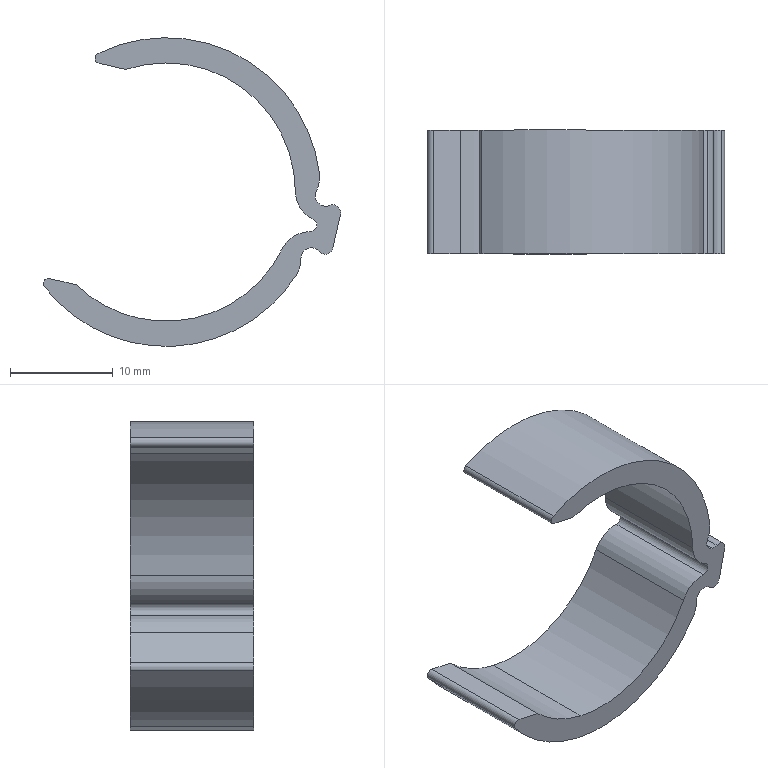Part | SolidWorks | features BaseBody 1 | 1 solid | 25 faces | box 28.907 x 12 x 30 mm | volume 1841 mm3 | cylinder 20 | plane 5 | commonest cylinder face diameters 6 x4 2 x3 25.1 x3 30 x3 1 x2 1.5 x2
STEP:
#1=CARTESIAN_POINT('',(1964.27,-217.65,847.477));
#2=VERTEX_POINT('',#1);
#3=CARTESIAN_POINT('',(1950.19,-217.65,840.769));
#4=VERTEX_POINT('',#3);
#5=CARTESIAN_POINT('',(1953.,-217.65,853.));
#6=DIRECTION('',(0.,1.,0.));
#7=DIRECTION('',(0.898,0.,-0.4401));
#8=AXIS2_PLACEMENT_3D('',#5,#6,#7);
#9=CIRCLE('',#8,12.55);
#10=EDGE_CURVE('',#2,#4,#9,.T.);
#11=ORIENTED_EDGE('',*,*,#10,.T.);
#12=CARTESIAN_POINT('',(1950.19,-229.65,840.769));
#13=VERTEX_POINT('',#12);
#14=CARTESIAN_POINT('',(1950.19,-217.65,840.769));
#15=DIRECTION('',(0.,-1.,0.));
#16=VECTOR('',#15,1000.);
#17=LINE('',#14,#16);
#18=EDGE_CURVE('',#4,#13,#17,.T.);
#19=ORIENTED_EDGE('',*,*,#18,.T.);
#20=CARTESIAN_POINT('',(1964.27,-229.65,847.477));
#21=VERTEX_POINT('',#20);
#22=CARTESIAN_POINT('',(1953.,-229.65,853.));
#23=DIRECTION('',(0.,1.,0.));
#24=DIRECTION('',(0.898,0.,-0.4401));
#25=AXIS2_PLACEMENT_3D('',#22,#23,#24);
#26=CIRCLE('',#25,12.55);
#27=EDGE_CURVE('',#21,#13,#26,.T.);
#28=ORIENTED_EDGE('',*,*,#27,.F.);
#29=CARTESIAN_POINT('',(1964.27,-229.65,847.477));
#30=DIRECTION('',(0.,1.,0.));
#31=VECTOR('',#30,1000.);
#32=LINE('',#29,#31);
#33=EDGE_CURVE('',#21,#2,#32,.T.);
#34=ORIENTED_EDGE('',*,*,#33,.T.);
#35=EDGE_LOOP('',(#11,#19,#28,#34));
#36=FACE_OUTER_BOUND('',#35,.T.);
#37=CARTESIAN_POINT('',(1953.,-217.65,853.));
#38=DIRECTION('',(0.,-1.,0.));
#39=DIRECTION('',(-0.2239,0.,-0.9746));
#40=AXIS2_PLACEMENT_3D('',#37,#38,#39);
#41=CYLINDRICAL_SURFACE('',#40,12.55);
#42=ADVANCED_FACE('',(#36),#41,.F.);
#43=CARTESIAN_POINT('',(1941.157,-217.65,843.795));
#44=VERTEX_POINT('',#43);
#45=CARTESIAN_POINT('',(1949.642,-217.65,838.381));
#46=VERTEX_POINT('',#45);
#47=CARTESIAN_POINT('',(1953.,-217.65,853.));
#48=DIRECTION('',(0.,-1.,0.));
#49=DIRECTION('',(-0.7895,0.,-0.6137));
#50=AXIS2_PLACEMENT_3D('',#47,#48,#49);
#51=CIRCLE('',#50,15.);
#52=EDGE_CURVE('',#44,#46,#51,.T.);
#53=ORIENTED_EDGE('',*,*,#52,.T.);
#54=CARTESIAN_POINT('',(1949.642,-229.65,838.381));
#55=VERTEX_POINT('',#54);
#56=CARTESIAN_POINT('',(1949.642,-217.65,838.381));
#57=DIRECTION('',(0.,-1.,0.));
#58=VECTOR('',#57,1000.);
#59=LINE('',#56,#58);
#60=EDGE_CURVE('',#46,#55,#59,.T.);
#61=ORIENTED_EDGE('',*,*,#60,.T.);
#62=CARTESIAN_POINT('',(1941.157,-229.65,843.795));
#63=VERTEX_POINT('',#62);
#64=CARTESIAN_POINT('',(1953.,-229.65,853.));
#65=DIRECTION('',(0.,-1.,0.));
#66=DIRECTION('',(-0.7895,0.,-0.6137));
#67=AXIS2_PLACEMENT_3D('',#64,#65,#66);
#68=CIRCLE('',#67,15.);
#69=EDGE_CURVE('',#63,#55,#68,.T.);
#70=ORIENTED_EDGE('',*,*,#69,.F.);
#71=CARTESIAN_POINT('',(1941.157,-229.65,843.795));
#72=DIRECTION('',(0.,1.,0.));
#73=VECTOR('',#72,1000.);
#74=LINE('',#71,#73);
#75=EDGE_CURVE('',#63,#44,#74,.T.);
#76=ORIENTED_EDGE('',*,*,#75,.T.);
#77=EDGE_LOOP('',(#53,#61,#70,#76));
#78=FACE_OUTER_BOUND('',#77,.T.);
#79=CARTESIAN_POINT('',(1953.,-217.65,853.));
#80=DIRECTION('',(0.,-1.,0.));
#81=DIRECTION('',(-0.2239,0.,-0.9746));
#82=AXIS2_PLACEMENT_3D('',#79,#80,#81);
#83=CYLINDRICAL_SURFACE('',#82,15.);
#84=ADVANCED_FACE('',(#78),#83,.T.);
#85=CARTESIAN_POINT('',(1968.258,-217.65,851.649));
#86=VERTEX_POINT('',#85);
#87=CARTESIAN_POINT('',(1968.885,-217.65,851.709));
#88=VERTEX_POINT('',#87);
#89=CARTESIAN_POINT('',(1968.482,-217.65,852.624));
#90=DIRECTION('',(0.,-1.,0.));
#91=DIRECTION('',(-0.892,0.,0.452));
#92=AXIS2_PLACEMENT_3D('',#89,#90,#91);
#93=CIRCLE('',#92,1.);
#94=EDGE_CURVE('',#86,#88,#93,.T.);
#95=ORIENTED_EDGE('',*,*,#94,.F.);
#96=CARTESIAN_POINT('',(1968.258,-229.65,851.649));
#97=VERTEX_POINT('',#96);
#98=CARTESIAN_POINT('',(1968.258,-230.85,851.649));
#99=DIRECTION('',(0.,-1.,0.));
#100=VECTOR('',#99,1000.);
#101=LINE('',#98,#100);
#102=EDGE_CURVE('',#86,#97,#101,.T.);
#103=ORIENTED_EDGE('',*,*,#102,.T.);
#104=CARTESIAN_POINT('',(1968.885,-229.65,851.709));
#105=VERTEX_POINT('',#104);
#106=CARTESIAN_POINT('',(1968.482,-229.65,852.624));
#107=DIRECTION('',(0.,1.,0.));
#108=DIRECTION('',(0.4028,0.,-0.9153));
#109=AXIS2_PLACEMENT_3D('',#106,#107,#108);
#110=CIRCLE('',#109,1.);
#111=EDGE_CURVE('',#105,#97,#110,.T.);
#112=ORIENTED_EDGE('',*,*,#111,.F.);
#113=CARTESIAN_POINT('',(1968.885,-217.65,851.709));
#114=DIRECTION('',(0.,-1.,0.));
#115=VECTOR('',#114,1000.);
#116=LINE('',#113,#115);
#117=EDGE_CURVE('',#88,#105,#116,.T.);
#118=ORIENTED_EDGE('',*,*,#117,.F.);
#119=EDGE_LOOP('',(#95,#103,#112,#118));
#120=FACE_OUTER_BOUND('',#119,.T.);
#121=CARTESIAN_POINT('',(1968.482,-230.85,852.624));
#122=DIRECTION('',(0.,-1.,0.));
#123=DIRECTION('',(-0.2239,0.,-0.9746));
#124=AXIS2_PLACEMENT_3D('',#121,#122,#123);
#125=CYLINDRICAL_SURFACE('',#124,1.);
#126=ADVANCED_FACE('',(#120),#125,.F.);
#127=CARTESIAN_POINT('',(1969.622,-217.65,851.633));
#128=VERTEX_POINT('',#127);
#129=CARTESIAN_POINT('',(1969.187,-217.65,851.022));
#130=DIRECTION('',(0.,1.,0.));
#131=DIRECTION('',(-0.4028,0.,0.9153));
#132=AXIS2_PLACEMENT_3D('',#129,#130,#131);
#133=CIRCLE('',#132,0.75);
#134=EDGE_CURVE('',#88,#128,#133,.T.);
#135=ORIENTED_EDGE('',*,*,#134,.T.);
#136=CARTESIAN_POINT('',(1969.938,-217.65,850.802));
#137=VERTEX_POINT('',#136);
#138=CARTESIAN_POINT('',(1969.158,-217.65,850.981));
#139=DIRECTION('',(0.,1.,0.));
#140=DIRECTION('',(0.5796,0.,0.8149));
#141=AXIS2_PLACEMENT_3D('',#138,#139,#140);
#142=CIRCLE('',#141,0.8);
#143=EDGE_CURVE('',#128,#137,#142,.T.);
#144=ORIENTED_EDGE('',*,*,#143,.T.);
#145=CARTESIAN_POINT('',(1969.199,-217.65,847.586));
#146=VERTEX_POINT('',#145);
#147=CARTESIAN_POINT('',(1969.199,-217.65,847.586));
#148=DIRECTION('',(0.2239,0.,0.9746));
#149=VECTOR('',#148,1000.);
#150=LINE('',#147,#149);
#151=EDGE_CURVE('',#146,#137,#150,.T.);
#152=ORIENTED_EDGE('',*,*,#151,.F.);
#153=CARTESIAN_POINT('',(1968.552,-217.65,846.976));
#154=VERTEX_POINT('',#153);
#155=CARTESIAN_POINT('',(1968.419,-217.65,847.765));
#156=DIRECTION('',(0.,1.,0.));
#157=DIRECTION('',(0.9746,0.,-0.2239));
#158=AXIS2_PLACEMENT_3D('',#155,#156,#157);
#159=CIRCLE('',#158,0.8);
#160=EDGE_CURVE('',#146,#154,#159,.T.);
#161=ORIENTED_EDGE('',*,*,#160,.T.);
#162=CARTESIAN_POINT('',(1967.856,-217.65,847.23));
#163=VERTEX_POINT('',#162);
#164=CARTESIAN_POINT('',(1968.428,-217.65,847.716));
#165=DIRECTION('',(0.,1.,0.));
#166=DIRECTION('',(0.1659,0.,-0.9861));
#167=AXIS2_PLACEMENT_3D('',#164,#165,#166);
#168=CIRCLE('',#167,0.75);
#169=EDGE_CURVE('',#154,#163,#168,.T.);
#170=ORIENTED_EDGE('',*,*,#169,.T.);
#171=CARTESIAN_POINT('',(1966.095,-217.65,846.565));
#172=VERTEX_POINT('',#171);
#173=CARTESIAN_POINT('',(1967.095,-217.65,846.582));
#174=DIRECTION('',(0.,-1.,0.));
#175=DIRECTION('',(0.7618,0.,0.6478));
#176=AXIS2_PLACEMENT_3D('',#173,#174,#175);
#177=CIRCLE('',#176,1.);
#178=EDGE_CURVE('',#163,#172,#177,.T.);
#179=ORIENTED_EDGE('',*,*,#178,.T.);
#180=CARTESIAN_POINT('',(1965.619,-217.65,844.891));
#181=VERTEX_POINT('',#180);
#182=CARTESIAN_POINT('',(1963.095,-217.65,846.513));
#183=DIRECTION('',(0.,1.,0.));
#184=DIRECTION('',(0.9998,0.,0.01744));
#185=AXIS2_PLACEMENT_3D('',#182,#183,#184);
#186=CIRCLE('',#185,3.);
#187=EDGE_CURVE('',#172,#181,#186,.T.);
#188=ORIENTED_EDGE('',*,*,#187,.T.);
#189=CARTESIAN_POINT('',(1953.,-217.65,853.));
#190=DIRECTION('',(0.,-1.,0.));
#191=DIRECTION('',(-0.7895,0.,-0.6137));
#192=AXIS2_PLACEMENT_3D('',#189,#190,#191);
#193=CIRCLE('',#192,15.);
#194=EDGE_CURVE('',#46,#181,#193,.T.);
#195=ORIENTED_EDGE('',*,*,#194,.F.);
#196=ORIENTED_EDGE('',*,*,#52,.F.);
#197=CARTESIAN_POINT('',(1941.663,-217.65,844.589));
#198=VERTEX_POINT('',#197);
#199=CARTESIAN_POINT('',(1941.552,-217.65,844.102));
#200=DIRECTION('',(0.,1.,0.));
#201=DIRECTION('',(-0.7895,0.,-0.6137));
#202=AXIS2_PLACEMENT_3D('',#199,#200,#201);
#203=CIRCLE('',#202,0.5);
#204=EDGE_CURVE('',#44,#198,#203,.T.);
#205=ORIENTED_EDGE('',*,*,#204,.T.);
#206=CARTESIAN_POINT('',(1944.262,-217.65,843.992));
#207=VERTEX_POINT('',#206);
#208=CARTESIAN_POINT('',(1944.262,-217.65,843.992));
#209=DIRECTION('',(-0.9746,0.,0.2239));
#210=VECTOR('',#209,1000.);
#211=LINE('',#208,#210);
#212=EDGE_CURVE('',#207,#198,#211,.T.);
#213=ORIENTED_EDGE('',*,*,#212,.F.);
#214=CARTESIAN_POINT('',(1953.,-217.65,853.));
#215=DIRECTION('',(0.,1.,0.));
#216=DIRECTION('',(0.898,0.,-0.4401));
#217=AXIS2_PLACEMENT_3D('',#214,#215,#216);
#218=CIRCLE('',#217,12.55);
#219=EDGE_CURVE('',#4,#207,#218,.T.);
#220=ORIENTED_EDGE('',*,*,#219,.F.);
#221=ORIENTED_EDGE('',*,*,#10,.F.);
#222=CARTESIAN_POINT('',(1967.002,-217.65,849.157));
#223=VERTEX_POINT('',#222);
#224=CARTESIAN_POINT('',(1966.963,-217.65,846.157));
#225=DIRECTION('',(0.,1.,0.));
#226=DIRECTION('',(-0.898,0.,0.4401));
#227=AXIS2_PLACEMENT_3D('',#224,#225,#226);
#228=CIRCLE('',#227,3.);
#229=EDGE_CURVE('',#2,#223,#228,.T.);
#230=ORIENTED_EDGE('',*,*,#229,.T.);
#231=CARTESIAN_POINT('',(1967.276,-217.65,850.348));
#232=VERTEX_POINT('',#231);
#233=CARTESIAN_POINT('',(1967.01,-217.65,849.782));
#234=DIRECTION('',(0.,-1.,0.));
#235=DIRECTION('',(-0.01288,0.,-0.9999));
#236=AXIS2_PLACEMENT_3D('',#233,#234,#235);
#237=CIRCLE('',#236,0.625);
#238=EDGE_CURVE('',#223,#232,#237,.T.);
#239=ORIENTED_EDGE('',*,*,#238,.T.);
#240=CARTESIAN_POINT('',(1965.55,-217.65,853.051));
#241=VERTEX_POINT('',#240);
#242=CARTESIAN_POINT('',(1968.55,-217.65,853.064));
#243=DIRECTION('',(0.,1.,0.));
#244=DIRECTION('',(-0.4247,0.,-0.9053));
#245=AXIS2_PLACEMENT_3D('',#242,#243,#244);
#246=CIRCLE('',#245,3.);
#247=EDGE_CURVE('',#232,#241,#246,.T.);
#248=ORIENTED_EDGE('',*,*,#247,.T.);
#249=CARTESIAN_POINT('',(1949.068,-217.65,864.918));
#250=VERTEX_POINT('',#249);
#251=CARTESIAN_POINT('',(1953.,-217.65,853.));
#252=DIRECTION('',(0.,1.,0.));
#253=DIRECTION('',(-0.3133,0.,0.9497));
#254=AXIS2_PLACEMENT_3D('',#251,#252,#253);
#255=CIRCLE('',#254,12.55);
#256=EDGE_CURVE('',#250,#241,#255,.T.);
#257=ORIENTED_EDGE('',*,*,#256,.F.);
#258=CARTESIAN_POINT('',(1946.47,-217.65,865.515));
#259=VERTEX_POINT('',#258);
#260=CARTESIAN_POINT('',(1946.47,-217.65,865.515));
#261=DIRECTION('',(0.9746,0.,-0.2239));
#262=VECTOR('',#261,1000.);
#263=LINE('',#260,#262);
#264=EDGE_CURVE('',#259,#250,#263,.T.);
#265=ORIENTED_EDGE('',*,*,#264,.F.);
#266=CARTESIAN_POINT('',(1946.361,-217.65,866.451));
#267=VERTEX_POINT('',#266);
#268=CARTESIAN_POINT('',(1946.582,-217.65,866.002));
#269=DIRECTION('',(0.,1.,0.));
#270=DIRECTION('',(-0.2239,0.,-0.9746));
#271=AXIS2_PLACEMENT_3D('',#268,#269,#270);
#272=CIRCLE('',#271,0.5);
#273=EDGE_CURVE('',#259,#267,#272,.T.);
#274=ORIENTED_EDGE('',*,*,#273,.T.);
#275=CARTESIAN_POINT('',(1967.893,-217.65,854.79));
#276=VERTEX_POINT('',#275);
#277=CARTESIAN_POINT('',(1953.,-217.65,853.));
#278=DIRECTION('',(0.,-1.,0.));
#279=DIRECTION('',(0.9929,0.,0.1193));
#280=AXIS2_PLACEMENT_3D('',#277,#278,#279);
#281=CIRCLE('',#280,15.);
#282=EDGE_CURVE('',#276,#267,#281,.T.);
#283=ORIENTED_EDGE('',*,*,#282,.F.);
#284=CARTESIAN_POINT('',(1967.59,-217.65,853.076));
#285=VERTEX_POINT('',#284);
#286=CARTESIAN_POINT('',(1964.914,-217.65,854.432));
#287=DIRECTION('',(0.,1.,0.));
#288=DIRECTION('',(0.9929,0.,0.1193));
#289=AXIS2_PLACEMENT_3D('',#286,#287,#288);
#290=CIRCLE('',#289,3.);
#291=EDGE_CURVE('',#276,#285,#290,.T.);
#292=ORIENTED_EDGE('',*,*,#291,.T.);
#293=CARTESIAN_POINT('',(1968.482,-217.65,852.624));
#294=DIRECTION('',(0.,-1.,0.));
#295=DIRECTION('',(-0.892,0.,0.452));
#296=AXIS2_PLACEMENT_3D('',#293,#294,#295);
#297=CIRCLE('',#296,1.);
#298=EDGE_CURVE('',#285,#86,#297,.T.);
#299=ORIENTED_EDGE('',*,*,#298,.T.);
#300=ORIENTED_EDGE('',*,*,#94,.T.);
#301=EDGE_LOOP('',(#135,#144,#152,#161,#170,#179,#188,#195,#196,#205,#213,#220,#221,#230,#239,#248,#257,#265,#274,#283,#292,#299,#300));
#302=FACE_OUTER_BOUND('',#301,.T.);
#303=CARTESIAN_POINT('',(1953.,-217.65,853.));
#304=DIRECTION('',(0.,-1.,0.));
#305=DIRECTION('',(-0.2239,0.,-0.9746));
#306=AXIS2_PLACEMENT_3D('',#303,#304,#305);
#307=PLANE('',#306);
#308=ADVANCED_FACE('',(#302),#307,.F.);
#309=ORIENTED_EDGE('',*,*,#102,.F.);
#310=ORIENTED_EDGE('',*,*,#298,.F.);
#311=CARTESIAN_POINT('',(1967.59,-229.65,853.076));
#312=VERTEX_POINT('',#311);
#313=CARTESIAN_POINT('',(1967.59,-229.65,853.076));
#314=DIRECTION('',(0.,1.,0.));
#315=VECTOR('',#314,1000.);
#316=LINE('',#313,#315);
#317=EDGE_CURVE('',#312,#285,#316,.T.);
#318=ORIENTED_EDGE('',*,*,#317,.F.);
#319=CARTESIAN_POINT('',(1968.482,-229.65,852.624));
#320=DIRECTION('',(0.,1.,0.));
#321=DIRECTION('',(0.4028,0.,-0.9153));
#322=AXIS2_PLACEMENT_3D('',#319,#320,#321);
#323=CIRCLE('',#322,1.);
#324=EDGE_CURVE('',#97,#312,#323,.T.);
#325=ORIENTED_EDGE('',*,*,#324,.F.);
#326=EDGE_LOOP('',(#309,#310,#318,#325));
#327=FACE_OUTER_BOUND('',#326,.T.);
#328=CARTESIAN_POINT('',(1968.482,-230.85,852.624));
#329=DIRECTION('',(0.,-1.,0.));
#330=DIRECTION('',(-0.2239,0.,-0.9746));
#331=AXIS2_PLACEMENT_3D('',#328,#329,#330);
#332=CYLINDRICAL_SURFACE('',#331,1.);
#333=ADVANCED_FACE('',(#327),#332,.F.);
#334=CARTESIAN_POINT('',(1969.622,-229.65,851.633));
#335=VERTEX_POINT('',#334);
#336=CARTESIAN_POINT('',(1969.187,-229.65,851.022));
#337=DIRECTION('',(0.,-1.,0.));
#338=DIRECTION('',(0.5796,0.,0.8149));
#339=AXIS2_PLACEMENT_3D('',#336,#337,#338);
#340=CIRCLE('',#339,0.75);
#341=EDGE_CURVE('',#335,#105,#340,.T.);
#342=ORIENTED_EDGE('',*,*,#341,.F.);
#343=CARTESIAN_POINT('',(1969.622,-217.65,851.633));
#344=DIRECTION('',(0.,-1.,0.));
#345=VECTOR('',#344,1000.);
#346=LINE('',#343,#345);
#347=EDGE_CURVE('',#128,#335,#346,.T.);
#348=ORIENTED_EDGE('',*,*,#347,.F.);
#349=ORIENTED_EDGE('',*,*,#134,.F.);
#350=ORIENTED_EDGE('',*,*,#117,.T.);
#351=EDGE_LOOP('',(#342,#348,#349,#350));
#352=FACE_OUTER_BOUND('',#351,.T.);
#353=CARTESIAN_POINT('',(1969.187,-217.516,851.022));
#354=DIRECTION('',(0.,-1.,0.));
#355=DIRECTION('',(-0.5796,0.,-0.8149));
#356=AXIS2_PLACEMENT_3D('',#353,#354,#355);
#357=CYLINDRICAL_SURFACE('',#356,0.75);
#358=ADVANCED_FACE('',(#352),#357,.T.);
#359=CARTESIAN_POINT('',(1969.938,-229.65,850.802));
#360=VERTEX_POINT('',#359);
#361=CARTESIAN_POINT('',(1969.938,-229.65,850.802));
#362=DIRECTION('',(0.,1.,0.));
#363=VECTOR('',#362,1000.);
#364=LINE('',#361,#363);
#365=EDGE_CURVE('',#360,#137,#364,.T.);
#366=ORIENTED_EDGE('',*,*,#365,.T.);
#367=ORIENTED_EDGE('',*,*,#143,.F.);
#368=ORIENTED_EDGE('',*,*,#347,.T.);
#369=CARTESIAN_POINT('',(1969.158,-229.65,850.981));
#370=DIRECTION('',(0.,-1.,0.));
#371=DIRECTION('',(0.9746,0.,-0.2239));
#372=AXIS2_PLACEMENT_3D('',#369,#370,#371);
#373=CIRCLE('',#372,0.8);
#374=EDGE_CURVE('',#360,#335,#373,.T.);
#375=ORIENTED_EDGE('',*,*,#374,.F.);
#376=EDGE_LOOP('',(#366,#367,#368,#375));
#377=FACE_OUTER_BOUND('',#376,.T.);
#378=CARTESIAN_POINT('',(1969.158,-229.806,850.981));
#379=DIRECTION('',(0.,1.,0.));
#380=DIRECTION('',(-0.2239,0.,-0.9746));
#381=AXIS2_PLACEMENT_3D('',#378,#379,#380);
#382=CYLINDRICAL_SURFACE('',#381,0.8);
#383=ADVANCED_FACE('',(#377),#382,.T.);
#384=CARTESIAN_POINT('',(1967.893,-229.65,854.79));
#385=VERTEX_POINT('',#384);
#386=CARTESIAN_POINT('',(1964.914,-229.65,854.432));
#387=DIRECTION('',(0.,-1.,0.));
#388=DIRECTION('',(0.892,0.,-0.452));
#389=AXIS2_PLACEMENT_3D('',#386,#387,#388);
#390=CIRCLE('',#389,3.);
#391=EDGE_CURVE('',#312,#385,#390,.T.);
#392=ORIENTED_EDGE('',*,*,#391,.T.);
#393=CARTESIAN_POINT('',(1946.361,-229.65,866.451));
#394=VERTEX_POINT('',#393);
#395=CARTESIAN_POINT('',(1953.,-229.65,853.));
#396=DIRECTION('',(0.,-1.,0.));
#397=DIRECTION('',(0.9929,0.,0.1193));
#398=AXIS2_PLACEMENT_3D('',#395,#396,#397);
#399=CIRCLE('',#398,15.);
#400=EDGE_CURVE('',#385,#394,#399,.T.);
#401=ORIENTED_EDGE('',*,*,#400,.T.);
#402=CARTESIAN_POINT('',(1946.47,-229.65,865.515));
#403=VERTEX_POINT('',#402);
#404=CARTESIAN_POINT('',(1946.582,-229.65,866.002));
#405=DIRECTION('',(0.,-1.,0.));
#406=DIRECTION('',(-0.4426,0.,0.8967));
#407=AXIS2_PLACEMENT_3D('',#404,#405,#406);
#408=CIRCLE('',#407,0.5);
#409=EDGE_CURVE('',#394,#403,#408,.T.);
#410=ORIENTED_EDGE('',*,*,#409,.T.);
#411=CARTESIAN_POINT('',(1949.068,-229.65,864.918));
#412=VERTEX_POINT('',#411);
#413=CARTESIAN_POINT('',(1946.47,-229.65,865.515));
#414=DIRECTION('',(0.9746,0.,-0.2239));
#415=VECTOR('',#414,1000.);
#416=LINE('',#413,#415);
#417=EDGE_CURVE('',#403,#412,#416,.T.);
#418=ORIENTED_EDGE('',*,*,#417,.T.);
#419=CARTESIAN_POINT('',(1965.55,-229.65,853.051));
#420=VERTEX_POINT('',#419);
#421=CARTESIAN_POINT('',(1953.,-229.65,853.));
#422=DIRECTION('',(0.,1.,0.));
#423=DIRECTION('',(-0.3133,0.,0.9497));
#424=AXIS2_PLACEMENT_3D('',#421,#422,#423);
#425=CIRCLE('',#424,12.55);
#426=EDGE_CURVE('',#412,#420,#425,.T.);
#427=ORIENTED_EDGE('',*,*,#426,.T.);
#428=CARTESIAN_POINT('',(1967.276,-229.65,850.348));
#429=VERTEX_POINT('',#428);
#430=CARTESIAN_POINT('',(1968.55,-229.65,853.064));
#431=DIRECTION('',(0.,-1.,0.));
#432=DIRECTION('',(-1.,0.,-0.004093));
#433=AXIS2_PLACEMENT_3D('',#430,#431,#432);
#434=CIRCLE('',#433,3.);
#435=EDGE_CURVE('',#420,#429,#434,.T.);
#436=ORIENTED_EDGE('',*,*,#435,.T.);
#437=CARTESIAN_POINT('',(1967.002,-229.65,849.157));
#438=VERTEX_POINT('',#437);
#439=CARTESIAN_POINT('',(1967.01,-229.65,849.782));
#440=DIRECTION('',(0.,-1.,0.));
#441=DIRECTION('',(-0.01288,0.,-0.9999));
#442=AXIS2_PLACEMENT_3D('',#439,#440,#441);
#443=CIRCLE('',#442,0.625);
#444=EDGE_CURVE('',#438,#429,#443,.T.);
#445=ORIENTED_EDGE('',*,*,#444,.F.);
#446=CARTESIAN_POINT('',(1966.963,-229.65,846.157));
#447=DIRECTION('',(0.,-1.,0.));
#448=DIRECTION('',(0.01288,0.,0.9999));
#449=AXIS2_PLACEMENT_3D('',#446,#447,#448);
#450=CIRCLE('',#449,3.);
#451=EDGE_CURVE('',#438,#21,#450,.T.);
#452=ORIENTED_EDGE('',*,*,#451,.T.);
#453=ORIENTED_EDGE('',*,*,#27,.T.);
#454=CARTESIAN_POINT('',(1944.262,-229.65,843.992));
#455=VERTEX_POINT('',#454);
#456=CARTESIAN_POINT('',(1953.,-229.65,853.));
#457=DIRECTION('',(0.,1.,0.));
#458=DIRECTION('',(0.898,0.,-0.4401));
#459=AXIS2_PLACEMENT_3D('',#456,#457,#458);
#460=CIRCLE('',#459,12.55);
#461=EDGE_CURVE('',#13,#455,#460,.T.);
#462=ORIENTED_EDGE('',*,*,#461,.T.);
#463=CARTESIAN_POINT('',(1941.663,-229.65,844.589));
#464=VERTEX_POINT('',#463);
#465=CARTESIAN_POINT('',(1944.262,-229.65,843.992));
#466=DIRECTION('',(-0.9746,0.,0.2239));
#467=VECTOR('',#466,1000.);
#468=LINE('',#465,#467);
#469=EDGE_CURVE('',#455,#464,#468,.T.);
#470=ORIENTED_EDGE('',*,*,#469,.T.);
#471=CARTESIAN_POINT('',(1941.552,-229.65,844.102));
#472=DIRECTION('',(0.,-1.,0.));
#473=DIRECTION('',(0.2239,0.,0.9746));
#474=AXIS2_PLACEMENT_3D('',#471,#472,#473);
#475=CIRCLE('',#474,0.5);
#476=EDGE_CURVE('',#464,#63,#475,.T.);
#477=ORIENTED_EDGE('',*,*,#476,.T.);
#478=ORIENTED_EDGE('',*,*,#69,.T.);
#479=CARTESIAN_POINT('',(1965.619,-229.65,844.891));
#480=VERTEX_POINT('',#479);
#481=CARTESIAN_POINT('',(1953.,-229.65,853.));
#482=DIRECTION('',(0.,-1.,0.));
#483=DIRECTION('',(-0.7895,0.,-0.6137));
#484=AXIS2_PLACEMENT_3D('',#481,#482,#483);
#485=CIRCLE('',#484,15.);
#486=EDGE_CURVE('',#55,#480,#485,.T.);
#487=ORIENTED_EDGE('',*,*,#486,.T.);
#488=CARTESIAN_POINT('',(1966.095,-229.65,846.565));
#489=VERTEX_POINT('',#488);
#490=CARTESIAN_POINT('',(1963.095,-229.65,846.513));
#491=DIRECTION('',(0.,-1.,0.));
#492=DIRECTION('',(0.8413,0.,-0.5406));
#493=AXIS2_PLACEMENT_3D('',#490,#491,#492);
#494=CIRCLE('',#493,3.);
#495=EDGE_CURVE('',#480,#489,#494,.T.);
#496=ORIENTED_EDGE('',*,*,#495,.T.);
#497=CARTESIAN_POINT('',(1967.856,-229.65,847.23));
#498=VERTEX_POINT('',#497);
#499=CARTESIAN_POINT('',(1967.095,-229.65,846.582));
#500=DIRECTION('',(0.,1.,0.));
#501=DIRECTION('',(-0.9998,0.,-0.01744));
#502=AXIS2_PLACEMENT_3D('',#499,#500,#501);
#503=CIRCLE('',#502,1.);
#504=EDGE_CURVE('',#489,#498,#503,.T.);
#505=ORIENTED_EDGE('',*,*,#504,.T.);
#506=CARTESIAN_POINT('',(1968.552,-229.65,846.976));
#507=VERTEX_POINT('',#506);
#508=CARTESIAN_POINT('',(1968.428,-229.65,847.716));
#509=DIRECTION('',(0.,-1.,0.));
#510=DIRECTION('',(-0.7618,0.,-0.6478));
#511=AXIS2_PLACEMENT_3D('',#508,#509,#510);
#512=CIRCLE('',#511,0.75);
#513=EDGE_CURVE('',#498,#507,#512,.T.);
#514=ORIENTED_EDGE('',*,*,#513,.T.);
#515=CARTESIAN_POINT('',(1969.199,-229.65,847.586));
#516=VERTEX_POINT('',#515);
#517=CARTESIAN_POINT('',(1968.419,-229.65,847.765));
#518=DIRECTION('',(0.,-1.,0.));
#519=DIRECTION('',(0.1659,0.,-0.9861));
#520=AXIS2_PLACEMENT_3D('',#517,#518,#519);
#521=CIRCLE('',#520,0.8);
#522=EDGE_CURVE('',#507,#516,#521,.T.);
#523=ORIENTED_EDGE('',*,*,#522,.T.);
#524=CARTESIAN_POINT('',(1969.199,-229.65,847.586));
#525=DIRECTION('',(0.2239,0.,0.9746));
#526=VECTOR('',#525,1000.);
#527=LINE('',#524,#526);
#528=EDGE_CURVE('',#516,#360,#527,.T.);
#529=ORIENTED_EDGE('',*,*,#528,.T.);
#530=ORIENTED_EDGE('',*,*,#374,.T.);
#531=ORIENTED_EDGE('',*,*,#341,.T.);
#532=ORIENTED_EDGE('',*,*,#111,.T.);
#533=ORIENTED_EDGE('',*,*,#324,.T.);
#534=EDGE_LOOP('',(#392,#401,#410,#418,#427,#436,#445,#452,#453,#462,#470,#477,#478,#487,#496,#505,#514,#523,#529,#530,#531,#532,#533));
#535=FACE_OUTER_BOUND('',#534,.T.);
#536=CARTESIAN_POINT('',(1953.,-229.65,853.));
#537=DIRECTION('',(0.,-1.,0.));
#538=DIRECTION('',(-0.2239,0.,-0.9746));
#539=AXIS2_PLACEMENT_3D('',#536,#537,#538);
#540=PLANE('',#539);
#541=ADVANCED_FACE('',(#535),#540,.T.);
#542=ORIENTED_EDGE('',*,*,#528,.F.);
#543=CARTESIAN_POINT('',(1969.199,-229.65,847.586));
#544=DIRECTION('',(0.,1.,0.));
#545=VECTOR('',#544,1000.);
#546=LINE('',#543,#545);
#547=EDGE_CURVE('',#516,#146,#546,.T.);
#548=ORIENTED_EDGE('',*,*,#547,.T.);
#549=ORIENTED_EDGE('',*,*,#151,.T.);
#550=ORIENTED_EDGE('',*,*,#365,.F.);
#551=EDGE_LOOP('',(#542,#548,#549,#550));
#552=FACE_OUTER_BOUND('',#551,.T.);
#553=CARTESIAN_POINT('',(1969.02,-217.65,846.806));
#554=DIRECTION('',(0.9746,0.,-0.2239));
#555=DIRECTION('',(-0.2239,0.,-0.9746));
#556=AXIS2_PLACEMENT_3D('',#553,#554,#555);
#557=PLANE('',#556);
#558=ADVANCED_FACE('',(#552),#557,.T.);
#559=CARTESIAN_POINT('',(1968.552,-229.65,846.976));
#560=DIRECTION('',(0.,1.,0.));
#561=VECTOR('',#560,1000.);
#562=LINE('',#559,#561);
#563=EDGE_CURVE('',#507,#154,#562,.T.);
#564=ORIENTED_EDGE('',*,*,#563,.T.);
#565=ORIENTED_EDGE('',*,*,#160,.F.);
#566=ORIENTED_EDGE('',*,*,#547,.F.);
#567=ORIENTED_EDGE('',*,*,#522,.F.);
#568=EDGE_LOOP('',(#564,#565,#566,#567));
#569=FACE_OUTER_BOUND('',#568,.T.);
#570=CARTESIAN_POINT('',(1968.419,-229.806,847.765));
#571=DIRECTION('',(0.,1.,0.));
#572=DIRECTION('',(-0.9746,0.,0.2239));
#573=AXIS2_PLACEMENT_3D('',#570,#571,#572);
#574=CYLINDRICAL_SURFACE('',#573,0.8);
#575=ADVANCED_FACE('',(#569),#574,.T.);
#576=ORIENTED_EDGE('',*,*,#169,.F.);
#577=ORIENTED_EDGE('',*,*,#563,.F.);
#578=ORIENTED_EDGE('',*,*,#513,.F.);
#579=CARTESIAN_POINT('',(1967.856,-229.65,847.23));
#580=DIRECTION('',(0.,1.,0.));
#581=VECTOR('',#580,1000.);
#582=LINE('',#579,#581);
#583=EDGE_CURVE('',#498,#163,#582,.T.);
#584=ORIENTED_EDGE('',*,*,#583,.T.);
#585=EDGE_LOOP('',(#576,#577,#578,#584));
#586=FACE_OUTER_BOUND('',#585,.T.);
#587=CARTESIAN_POINT('',(1968.428,-229.801,847.716));
#588=DIRECTION('',(0.,1.,0.));
#589=DIRECTION('',(-0.1659,0.,0.9861));
#590=AXIS2_PLACEMENT_3D('',#587,#588,#589);
#591=CYLINDRICAL_SURFACE('',#590,0.75);
#592=ADVANCED_FACE('',(#586),#591,.T.);
#593=CARTESIAN_POINT('',(1966.095,-217.65,846.565));
#594=DIRECTION('',(0.,-1.,0.));
#595=VECTOR('',#594,1000.);
#596=LINE('',#593,#595);
#597=EDGE_CURVE('',#172,#489,#596,.T.);
#598=ORIENTED_EDGE('',*,*,#597,.F.);
#599=ORIENTED_EDGE('',*,*,#178,.F.);
#600=ORIENTED_EDGE('',*,*,#583,.F.);
#601=ORIENTED_EDGE('',*,*,#504,.F.);
#602=EDGE_LOOP('',(#598,#599,#600,#601));
#603=FACE_OUTER_BOUND('',#602,.T.);
#604=CARTESIAN_POINT('',(1967.095,-230.85,846.582));
#605=DIRECTION('',(0.,-1.,0.));
#606=DIRECTION('',(-0.2239,0.,-0.9746));
#607=AXIS2_PLACEMENT_3D('',#604,#605,#606);
#608=CYLINDRICAL_SURFACE('',#607,1.);
#609=ADVANCED_FACE('',(#603),#608,.F.);
#610=ORIENTED_EDGE('',*,*,#495,.F.);
#611=CARTESIAN_POINT('',(1965.619,-217.65,844.891));
#612=DIRECTION('',(0.,-1.,0.));
#613=VECTOR('',#612,1000.);
#614=LINE('',#611,#613);
#615=EDGE_CURVE('',#181,#480,#614,.T.);
#616=ORIENTED_EDGE('',*,*,#615,.F.);
#617=ORIENTED_EDGE('',*,*,#187,.F.);
#618=ORIENTED_EDGE('',*,*,#597,.T.);
#619=EDGE_LOOP('',(#610,#616,#617,#618));
#620=FACE_OUTER_BOUND('',#619,.T.);
#621=CARTESIAN_POINT('',(1963.095,-217.516,846.513));
#622=DIRECTION('',(0.,-1.,0.));
#623=DIRECTION('',(-0.8413,0.,0.5406));
#624=AXIS2_PLACEMENT_3D('',#621,#622,#623);
#625=CYLINDRICAL_SURFACE('',#624,3.);
#626=ADVANCED_FACE('',(#620),#625,.T.);
#627=ORIENTED_EDGE('',*,*,#60,.F.);
#628=ORIENTED_EDGE('',*,*,#194,.T.);
#629=ORIENTED_EDGE('',*,*,#615,.T.);
#630=ORIENTED_EDGE('',*,*,#486,.F.);
#631=EDGE_LOOP('',(#627,#628,#629,#630));
#632=FACE_OUTER_BOUND('',#631,.T.);
#633=CARTESIAN_POINT('',(1953.,-217.65,853.));
#634=DIRECTION('',(0.,-1.,0.));
#635=DIRECTION('',(-0.2239,0.,-0.9746));
#636=AXIS2_PLACEMENT_3D('',#633,#634,#635);
#637=CYLINDRICAL_SURFACE('',#636,15.);
#638=ADVANCED_FACE('',(#632),#637,.T.);
#639=ORIENTED_EDGE('',*,*,#204,.F.);
#640=ORIENTED_EDGE('',*,*,#75,.F.);
#641=ORIENTED_EDGE('',*,*,#476,.F.);
#642=CARTESIAN_POINT('',(1941.663,-229.65,844.589));
#643=DIRECTION('',(0.,1.,0.));
#644=VECTOR('',#643,1000.);
#645=LINE('',#642,#644);
#646=EDGE_CURVE('',#464,#198,#645,.T.);
#647=ORIENTED_EDGE('',*,*,#646,.T.);
#648=EDGE_LOOP('',(#639,#640,#641,#647));
#649=FACE_OUTER_BOUND('',#648,.T.);
#650=CARTESIAN_POINT('',(1941.552,-229.806,844.102));
#651=DIRECTION('',(0.,1.,0.));
#652=DIRECTION('',(0.7895,0.,0.6137));
#653=AXIS2_PLACEMENT_3D('',#650,#651,#652);
#654=CYLINDRICAL_SURFACE('',#653,0.5);
#655=ADVANCED_FACE('',(#649),#654,.T.);
#656=ORIENTED_EDGE('',*,*,#469,.F.);
#657=CARTESIAN_POINT('',(1944.262,-217.65,843.992));
#658=DIRECTION('',(0.,-1.,0.));
#659=VECTOR('',#658,1000.);
#660=LINE('',#657,#659);
#661=EDGE_CURVE('',#207,#455,#660,.T.);
#662=ORIENTED_EDGE('',*,*,#661,.F.);
#663=ORIENTED_EDGE('',*,*,#212,.T.);
#664=ORIENTED_EDGE('',*,*,#646,.F.);
#665=EDGE_LOOP('',(#656,#662,#663,#664));
#666=FACE_OUTER_BOUND('',#665,.T.);
#667=CARTESIAN_POINT('',(1944.262,-217.65,843.992));
#668=DIRECTION('',(0.2239,0.,0.9746));
#669=DIRECTION('',(0.9746,0.,-0.2239));
#670=AXIS2_PLACEMENT_3D('',#667,#668,#669);
#671=PLANE('',#670);
#672=ADVANCED_FACE('',(#666),#671,.T.);
#673=ORIENTED_EDGE('',*,*,#18,.F.);
#674=ORIENTED_EDGE('',*,*,#219,.T.);
#675=ORIENTED_EDGE('',*,*,#661,.T.);
#676=ORIENTED_EDGE('',*,*,#461,.F.);
#677=EDGE_LOOP('',(#673,#674,#675,#676));
#678=FACE_OUTER_BOUND('',#677,.T.);
#679=CARTESIAN_POINT('',(1953.,-217.65,853.));
#680=DIRECTION('',(0.,-1.,0.));
#681=DIRECTION('',(-0.2239,0.,-0.9746));
#682=AXIS2_PLACEMENT_3D('',#679,#680,#681);
#683=CYLINDRICAL_SURFACE('',#682,12.55);
#684=ADVANCED_FACE('',(#678),#683,.F.);
#685=ORIENTED_EDGE('',*,*,#229,.F.);
#686=ORIENTED_EDGE('',*,*,#33,.F.);
#687=ORIENTED_EDGE('',*,*,#451,.F.);
#688=CARTESIAN_POINT('',(1967.002,-229.65,849.157));
#689=DIRECTION('',(0.,1.,0.));
#690=VECTOR('',#689,1000.);
#691=LINE('',#688,#690);
#692=EDGE_CURVE('',#438,#223,#691,.T.);
#693=ORIENTED_EDGE('',*,*,#692,.T.);
#694=EDGE_LOOP('',(#685,#686,#687,#693));
#695=FACE_OUTER_BOUND('',#694,.T.);
#696=CARTESIAN_POINT('',(1966.963,-229.806,846.157));
#697=DIRECTION('',(0.,1.,0.));
#698=DIRECTION('',(0.898,0.,-0.4401));
#699=AXIS2_PLACEMENT_3D('',#696,#697,#698);
#700=CYLINDRICAL_SURFACE('',#699,3.);
#701=ADVANCED_FACE('',(#695),#700,.T.);
#702=ORIENTED_EDGE('',*,*,#444,.T.);
#703=CARTESIAN_POINT('',(1967.276,-217.65,850.348));
#704=DIRECTION('',(0.,-1.,0.));
#705=VECTOR('',#704,1000.);
#706=LINE('',#703,#705);
#707=EDGE_CURVE('',#232,#429,#706,.T.);
#708=ORIENTED_EDGE('',*,*,#707,.F.);
#709=ORIENTED_EDGE('',*,*,#238,.F.);
#710=ORIENTED_EDGE('',*,*,#692,.F.);
#711=EDGE_LOOP('',(#702,#708,#709,#710));
#712=FACE_OUTER_BOUND('',#711,.T.);
#713=CARTESIAN_POINT('',(1967.01,-230.85,849.782));
#714=DIRECTION('',(0.,-1.,0.));
#715=DIRECTION('',(-0.2239,0.,-0.9746));
#716=AXIS2_PLACEMENT_3D('',#713,#714,#715);
#717=CYLINDRICAL_SURFACE('',#716,0.625);
#718=ADVANCED_FACE('',(#712),#717,.F.);
#719=ORIENTED_EDGE('',*,*,#435,.F.);
#720=CARTESIAN_POINT('',(1965.55,-217.65,853.051));
#721=DIRECTION('',(0.,-1.,0.));
#722=VECTOR('',#721,1000.);
#723=LINE('',#720,#722);
#724=EDGE_CURVE('',#241,#420,#723,.T.);
#725=ORIENTED_EDGE('',*,*,#724,.F.);
#726=ORIENTED_EDGE('',*,*,#247,.F.);
#727=ORIENTED_EDGE('',*,*,#707,.T.);
#728=EDGE_LOOP('',(#719,#725,#726,#727));
#729=FACE_OUTER_BOUND('',#728,.T.);
#730=CARTESIAN_POINT('',(1968.55,-217.516,853.064));
#731=DIRECTION('',(0.,-1.,0.));
#732=DIRECTION('',(1.,0.,0.004093));
#733=AXIS2_PLACEMENT_3D('',#730,#731,#732);
#734=CYLINDRICAL_SURFACE('',#733,3.);
#735=ADVANCED_FACE('',(#729),#734,.T.);
#736=ORIENTED_EDGE('',*,*,#724,.T.);
#737=ORIENTED_EDGE('',*,*,#426,.F.);
#738=CARTESIAN_POINT('',(1949.068,-217.65,864.918));
#739=DIRECTION('',(0.,-1.,0.));
#740=VECTOR('',#739,1000.);
#741=LINE('',#738,#740);
#742=EDGE_CURVE('',#250,#412,#741,.T.);
#743=ORIENTED_EDGE('',*,*,#742,.F.);
#744=ORIENTED_EDGE('',*,*,#256,.T.);
#745=EDGE_LOOP('',(#736,#737,#743,#744));
#746=FACE_OUTER_BOUND('',#745,.T.);
#747=CARTESIAN_POINT('',(1953.,-217.65,853.));
#748=DIRECTION('',(0.,-1.,0.));
#749=DIRECTION('',(-0.2239,0.,-0.9746));
#750=AXIS2_PLACEMENT_3D('',#747,#748,#749);
#751=CYLINDRICAL_SURFACE('',#750,12.55);
#752=ADVANCED_FACE('',(#746),#751,.F.);
#753=ORIENTED_EDGE('',*,*,#264,.T.);
#754=ORIENTED_EDGE('',*,*,#742,.T.);
#755=ORIENTED_EDGE('',*,*,#417,.F.);
#756=CARTESIAN_POINT('',(1946.47,-229.65,865.515));
#757=DIRECTION('',(0.,1.,0.));
#758=VECTOR('',#757,1000.);
#759=LINE('',#756,#758);
#760=EDGE_CURVE('',#403,#259,#759,.T.);
#761=ORIENTED_EDGE('',*,*,#760,.T.);
#762=EDGE_LOOP('',(#753,#754,#755,#761));
#763=FACE_OUTER_BOUND('',#762,.T.);
#764=CARTESIAN_POINT('',(1945.193,-217.65,865.808));
#765=DIRECTION('',(-0.2239,0.,-0.9746));
#766=DIRECTION('',(-0.9746,0.,0.2239));
#767=AXIS2_PLACEMENT_3D('',#764,#765,#766);
#768=PLANE('',#767);
#769=ADVANCED_FACE('',(#763),#768,.T.);
#770=ORIENTED_EDGE('',*,*,#273,.F.);
#771=ORIENTED_EDGE('',*,*,#760,.F.);
#772=ORIENTED_EDGE('',*,*,#409,.F.);
#773=CARTESIAN_POINT('',(1946.361,-229.65,866.451));
#774=DIRECTION('',(0.,1.,0.));
#775=VECTOR('',#774,1000.);
#776=LINE('',#773,#775);
#777=EDGE_CURVE('',#394,#267,#776,.T.);
#778=ORIENTED_EDGE('',*,*,#777,.T.);
#779=EDGE_LOOP('',(#770,#771,#772,#778));
#780=FACE_OUTER_BOUND('',#779,.T.);
#781=CARTESIAN_POINT('',(1946.582,-229.806,866.002));
#782=DIRECTION('',(0.,1.,0.));
#783=DIRECTION('',(0.2239,0.,0.9746));
#784=AXIS2_PLACEMENT_3D('',#781,#782,#783);
#785=CYLINDRICAL_SURFACE('',#784,0.5);
#786=ADVANCED_FACE('',(#780),#785,.T.);
#787=ORIENTED_EDGE('',*,*,#282,.T.);
#788=ORIENTED_EDGE('',*,*,#777,.F.);
#789=ORIENTED_EDGE('',*,*,#400,.F.);
#790=CARTESIAN_POINT('',(1967.893,-229.65,854.79));
#791=DIRECTION('',(0.,1.,0.));
#792=VECTOR('',#791,1000.);
#793=LINE('',#790,#792);
#794=EDGE_CURVE('',#385,#276,#793,.T.);
#795=ORIENTED_EDGE('',*,*,#794,.T.);
#796=EDGE_LOOP('',(#787,#788,#789,#795));
#797=FACE_OUTER_BOUND('',#796,.T.);
#798=CARTESIAN_POINT('',(1953.,-217.65,853.));
#799=DIRECTION('',(0.,-1.,0.));
#800=DIRECTION('',(-0.2239,0.,-0.9746));
#801=AXIS2_PLACEMENT_3D('',#798,#799,#800);
#802=CYLINDRICAL_SURFACE('',#801,15.);
#803=ADVANCED_FACE('',(#797),#802,.T.);
#804=ORIENTED_EDGE('',*,*,#291,.F.);
#805=ORIENTED_EDGE('',*,*,#794,.F.);
#806=ORIENTED_EDGE('',*,*,#391,.F.);
#807=ORIENTED_EDGE('',*,*,#317,.T.);
#808=EDGE_LOOP('',(#804,#805,#806,#807));
#809=FACE_OUTER_BOUND('',#808,.T.);
#810=CARTESIAN_POINT('',(1964.914,-229.806,854.432));
#811=DIRECTION('',(0.,1.,0.));
#812=DIRECTION('',(-0.9929,0.,-0.1193));
#813=AXIS2_PLACEMENT_3D('',#810,#811,#812);
#814=CYLINDRICAL_SURFACE('',#813,3.);
#815=ADVANCED_FACE('',(#809),#814,.T.);
#816=CLOSED_SHELL('',(#42,#84,#126,#308,#333,#358,#383,#541,#558,#575,#592,#609,#626,#638,#655,#672,#684,#701,#718,#735,#752,#769,#786,#803,#815));
#817=MANIFOLD_SOLID_BREP('',#816);
#818=CARTESIAN_POINT('',(0.,0.,0.));
#819=DIRECTION('',(0.,0.,1.));
#820=DIRECTION('',(1.,0.,0.));
#821=AXIS2_PLACEMENT_3D('',#818,#819,#820);
#822=(LENGTH_UNIT()NAMED_UNIT(*)SI_UNIT(.MILLI.,.METRE.));
#823=UNCERTAINTY_MEASURE_WITH_UNIT(LENGTH_MEASURE(0.00001),#822,'','');
#824=(NAMED_UNIT(*)PLANE_ANGLE_UNIT()SI_UNIT($,.RADIAN.));
#825=(NAMED_UNIT(*)SI_UNIT($,.STERADIAN.)SOLID_ANGLE_UNIT());
#826=(GEOMETRIC_REPRESENTATION_CONTEXT(3)GLOBAL_UNCERTAINTY_ASSIGNED_CONTEXT((#823))GLOBAL_UNIT_ASSIGNED_CONTEXT((#822,#824,#825))REPRESENTATION_CONTEXT('',''));
#827=ADVANCED_BREP_SHAPE_REPRESENTATION('',(#817,#821),#826);